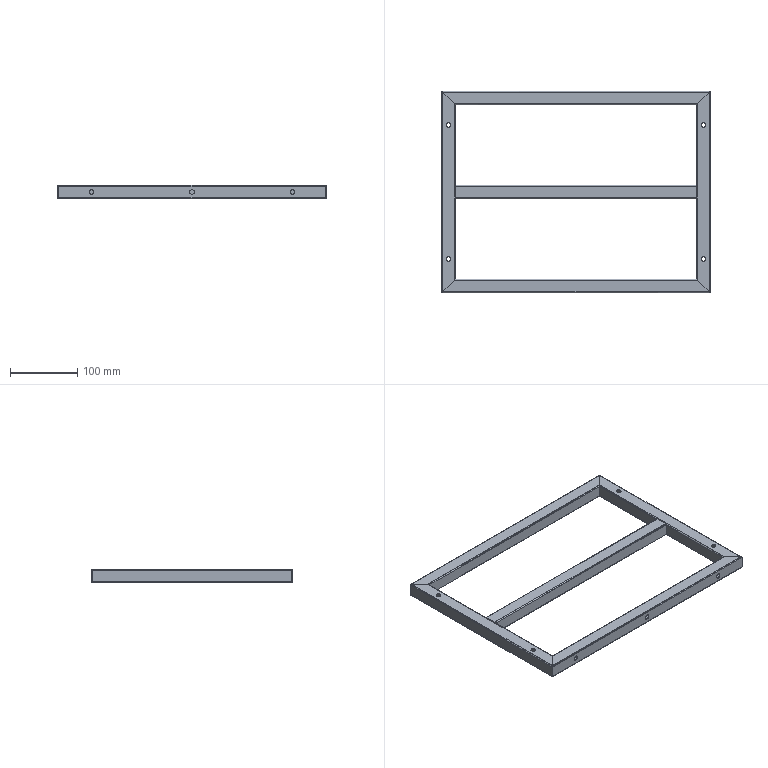Part | SolidWorks | features Cut 2, ICE 1, WeldMemberFeat 1, WeldmentFeature 1 | 5 solids | 122 faces | box 400 x 300 x 20 mm | volume 147653 mm3 | cylinder 72 | plane 50 | commonest cylinder face diameters 7 x28 0.6 x20 3 x20 10 x4